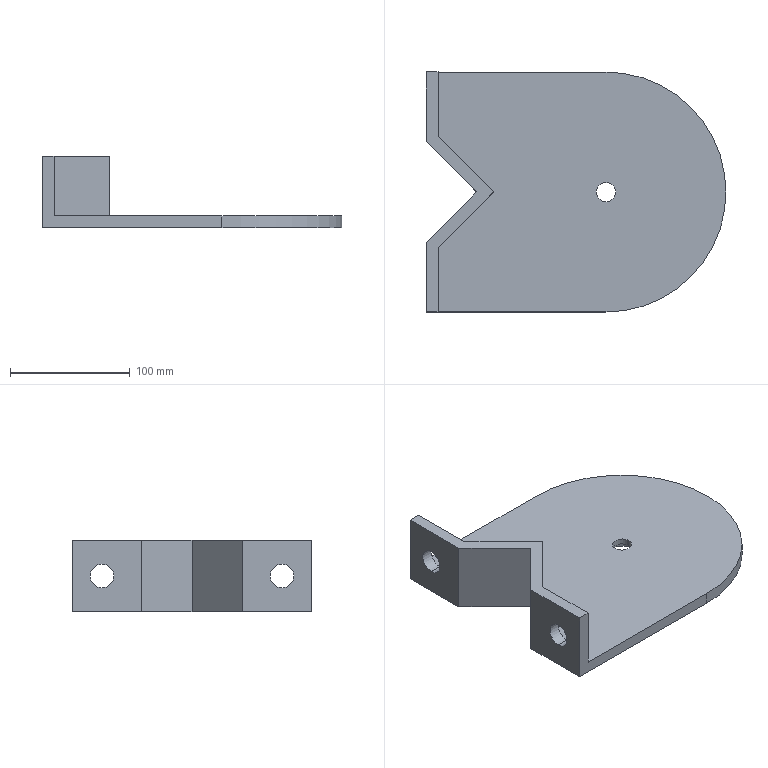Part | SolidWorks | features ICE 3, Cut 1, Extrusion 1 | 1 solid | 23 faces | box 250 x 200 x 60 mm | volume 547961 mm3 | plane 14 | cylinder 9 | commonest cylinder face diameters 20 x4 16 x2 24 x2 200 x1
STEP:
#1=CARTESIAN_POINT('',(12.,0.,5.));
#2=VERTEX_POINT('',#1);
#3=CARTESIAN_POINT('',(-12.,0.,5.));
#4=VERTEX_POINT('',#3);
#5=CARTESIAN_POINT('',(0.,0.,5.));
#6=DIRECTION('',(0.,0.,-1.));
#7=DIRECTION('',(-1.,0.,0.));
#8=AXIS2_PLACEMENT_3D('',#5,#6,#7);
#9=CIRCLE('',#8,12.);
#10=EDGE_CURVE('',#2,#4,#9,.T.);
#11=ORIENTED_EDGE('',*,*,#10,.F.);
#12=CARTESIAN_POINT('',(12.,0.,0.));
#13=VERTEX_POINT('',#12);
#14=CARTESIAN_POINT('',(12.,0.,5.));
#15=DIRECTION('',(0.,0.,-1.));
#16=VECTOR('',#15,1000.);
#17=LINE('',#14,#16);
#18=EDGE_CURVE('',#2,#13,#17,.T.);
#19=ORIENTED_EDGE('',*,*,#18,.T.);
#20=CARTESIAN_POINT('',(-12.,0.,0.));
#21=VERTEX_POINT('',#20);
#22=CARTESIAN_POINT('',(0.,0.,0.));
#23=DIRECTION('',(0.,0.,-1.));
#24=DIRECTION('',(-1.,0.,0.));
#25=AXIS2_PLACEMENT_3D('',#22,#23,#24);
#26=CIRCLE('',#25,12.);
#27=EDGE_CURVE('',#13,#21,#26,.T.);
#28=ORIENTED_EDGE('',*,*,#27,.T.);
#29=CARTESIAN_POINT('',(-12.,0.,5.));
#30=DIRECTION('',(0.,0.,-1.));
#31=VECTOR('',#30,1000.);
#32=LINE('',#29,#31);
#33=EDGE_CURVE('',#4,#21,#32,.T.);
#34=ORIENTED_EDGE('',*,*,#33,.F.);
#35=EDGE_LOOP('',(#11,#19,#28,#34));
#36=FACE_OUTER_BOUND('',#35,.T.);
#37=CARTESIAN_POINT('',(0.,0.,5.));
#38=DIRECTION('',(0.,0.,-1.));
#39=DIRECTION('',(-1.,0.,0.));
#40=AXIS2_PLACEMENT_3D('',#37,#38,#39);
#41=CYLINDRICAL_SURFACE('',#40,12.);
#42=ADVANCED_FACE('',(#36),#41,.F.);
#43=CARTESIAN_POINT('',(-140.,-75.,20.));
#44=VERTEX_POINT('',#43);
#45=CARTESIAN_POINT('',(-140.,-75.,40.));
#46=VERTEX_POINT('',#45);
#47=CARTESIAN_POINT('',(-140.,-75.,30.));
#48=DIRECTION('',(-1.,0.,0.));
#49=DIRECTION('',(0.,0.,1.));
#50=AXIS2_PLACEMENT_3D('',#47,#48,#49);
#51=CIRCLE('',#50,10.);
#52=EDGE_CURVE('',#44,#46,#51,.T.);
#53=ORIENTED_EDGE('',*,*,#52,.F.);
#54=CARTESIAN_POINT('',(-150.,-75.,20.));
#55=VERTEX_POINT('',#54);
#56=CARTESIAN_POINT('',(-110.,-75.,20.));
#57=DIRECTION('',(-1.,0.,0.));
#58=VECTOR('',#57,1000.);
#59=LINE('',#56,#58);
#60=EDGE_CURVE('',#44,#55,#59,.T.);
#61=ORIENTED_EDGE('',*,*,#60,.T.);
#62=CARTESIAN_POINT('',(-150.,-75.,40.));
#63=VERTEX_POINT('',#62);
#64=CARTESIAN_POINT('',(-150.,-75.,30.));
#65=DIRECTION('',(-1.,0.,0.));
#66=DIRECTION('',(0.,0.,1.));
#67=AXIS2_PLACEMENT_3D('',#64,#65,#66);
#68=CIRCLE('',#67,10.);
#69=EDGE_CURVE('',#55,#63,#68,.T.);
#70=ORIENTED_EDGE('',*,*,#69,.T.);
#71=CARTESIAN_POINT('',(-110.,-75.,40.));
#72=DIRECTION('',(-1.,0.,0.));
#73=VECTOR('',#72,1000.);
#74=LINE('',#71,#73);
#75=EDGE_CURVE('',#46,#63,#74,.T.);
#76=ORIENTED_EDGE('',*,*,#75,.F.);
#77=EDGE_LOOP('',(#53,#61,#70,#76));
#78=FACE_OUTER_BOUND('',#77,.T.);
#79=CARTESIAN_POINT('',(-110.,-75.,30.));
#80=DIRECTION('',(-1.,0.,0.));
#81=DIRECTION('',(0.,0.,1.));
#82=AXIS2_PLACEMENT_3D('',#79,#80,#81);
#83=CYLINDRICAL_SURFACE('',#82,10.);
#84=ADVANCED_FACE('',(#78),#83,.F.);
#85=CARTESIAN_POINT('',(-140.,75.,20.));
#86=VERTEX_POINT('',#85);
#87=CARTESIAN_POINT('',(-140.,75.,40.));
#88=VERTEX_POINT('',#87);
#89=CARTESIAN_POINT('',(-140.,75.,30.));
#90=DIRECTION('',(-1.,0.,0.));
#91=DIRECTION('',(0.,0.,1.));
#92=AXIS2_PLACEMENT_3D('',#89,#90,#91);
#93=CIRCLE('',#92,10.);
#94=EDGE_CURVE('',#86,#88,#93,.T.);
#95=ORIENTED_EDGE('',*,*,#94,.F.);
#96=CARTESIAN_POINT('',(-150.,75.,20.));
#97=VERTEX_POINT('',#96);
#98=CARTESIAN_POINT('',(-110.,75.,20.));
#99=DIRECTION('',(-1.,0.,0.));
#100=VECTOR('',#99,1000.);
#101=LINE('',#98,#100);
#102=EDGE_CURVE('',#86,#97,#101,.T.);
#103=ORIENTED_EDGE('',*,*,#102,.T.);
#104=CARTESIAN_POINT('',(-150.,75.,40.));
#105=VERTEX_POINT('',#104);
#106=CARTESIAN_POINT('',(-150.,75.,30.));
#107=DIRECTION('',(-1.,0.,0.));
#108=DIRECTION('',(0.,0.,1.));
#109=AXIS2_PLACEMENT_3D('',#106,#107,#108);
#110=CIRCLE('',#109,10.);
#111=EDGE_CURVE('',#97,#105,#110,.T.);
#112=ORIENTED_EDGE('',*,*,#111,.T.);
#113=CARTESIAN_POINT('',(-110.,75.,40.));
#114=DIRECTION('',(-1.,0.,0.));
#115=VECTOR('',#114,1000.);
#116=LINE('',#113,#115);
#117=EDGE_CURVE('',#88,#105,#116,.T.);
#118=ORIENTED_EDGE('',*,*,#117,.F.);
#119=EDGE_LOOP('',(#95,#103,#112,#118));
#120=FACE_OUTER_BOUND('',#119,.T.);
#121=CARTESIAN_POINT('',(-110.,75.,30.));
#122=DIRECTION('',(-1.,0.,0.));
#123=DIRECTION('',(0.,0.,1.));
#124=AXIS2_PLACEMENT_3D('',#121,#122,#123);
#125=CYLINDRICAL_SURFACE('',#124,10.);
#126=ADVANCED_FACE('',(#120),#125,.F.);
#127=CARTESIAN_POINT('',(-8.,0.,10.));
#128=VERTEX_POINT('',#127);
#129=CARTESIAN_POINT('',(8.,0.,10.));
#130=VERTEX_POINT('',#129);
#131=CARTESIAN_POINT('',(0.,0.,10.));
#132=DIRECTION('',(0.,0.,1.));
#133=DIRECTION('',(1.,0.,0.));
#134=AXIS2_PLACEMENT_3D('',#131,#132,#133);
#135=CIRCLE('',#134,8.);
#136=EDGE_CURVE('',#128,#130,#135,.T.);
#137=ORIENTED_EDGE('',*,*,#136,.T.);
#138=CARTESIAN_POINT('',(8.,0.,5.));
#139=VERTEX_POINT('',#138);
#140=CARTESIAN_POINT('',(8.,0.,10.));
#141=DIRECTION('',(0.,0.,-1.));
#142=VECTOR('',#141,1000.);
#143=LINE('',#140,#142);
#144=EDGE_CURVE('',#130,#139,#143,.T.);
#145=ORIENTED_EDGE('',*,*,#144,.T.);
#146=CARTESIAN_POINT('',(-8.,0.,5.));
#147=VERTEX_POINT('',#146);
#148=CARTESIAN_POINT('',(0.,0.,5.));
#149=DIRECTION('',(0.,0.,-1.));
#150=DIRECTION('',(-1.,0.,0.));
#151=AXIS2_PLACEMENT_3D('',#148,#149,#150);
#152=CIRCLE('',#151,8.);
#153=EDGE_CURVE('',#139,#147,#152,.T.);
#154=ORIENTED_EDGE('',*,*,#153,.T.);
#155=CARTESIAN_POINT('',(-8.,0.,10.));
#156=DIRECTION('',(0.,0.,-1.));
#157=VECTOR('',#156,1000.);
#158=LINE('',#155,#157);
#159=EDGE_CURVE('',#128,#147,#158,.T.);
#160=ORIENTED_EDGE('',*,*,#159,.F.);
#161=EDGE_LOOP('',(#137,#145,#154,#160));
#162=FACE_OUTER_BOUND('',#161,.T.);
#163=CARTESIAN_POINT('',(0.,0.,10.));
#164=DIRECTION('',(0.,0.,-1.));
#165=DIRECTION('',(-1.,0.,0.));
#166=AXIS2_PLACEMENT_3D('',#163,#164,#165);
#167=CYLINDRICAL_SURFACE('',#166,8.);
#168=ADVANCED_FACE('',(#162),#167,.F.);
#169=ORIENTED_EDGE('',*,*,#144,.F.);
#170=CARTESIAN_POINT('',(0.,0.,10.));
#171=DIRECTION('',(0.,0.,1.));
#172=DIRECTION('',(1.,0.,0.));
#173=AXIS2_PLACEMENT_3D('',#170,#171,#172);
#174=CIRCLE('',#173,8.);
#175=EDGE_CURVE('',#130,#128,#174,.T.);
#176=ORIENTED_EDGE('',*,*,#175,.T.);
#177=ORIENTED_EDGE('',*,*,#159,.T.);
#178=CARTESIAN_POINT('',(0.,0.,5.));
#179=DIRECTION('',(0.,0.,-1.));
#180=DIRECTION('',(-1.,0.,0.));
#181=AXIS2_PLACEMENT_3D('',#178,#179,#180);
#182=CIRCLE('',#181,8.);
#183=EDGE_CURVE('',#147,#139,#182,.T.);
#184=ORIENTED_EDGE('',*,*,#183,.T.);
#185=EDGE_LOOP('',(#169,#176,#177,#184));
#186=FACE_OUTER_BOUND('',#185,.T.);
#187=CARTESIAN_POINT('',(0.,0.,10.));
#188=DIRECTION('',(0.,0.,-1.));
#189=DIRECTION('',(-1.,0.,0.));
#190=AXIS2_PLACEMENT_3D('',#187,#188,#189);
#191=CYLINDRICAL_SURFACE('',#190,8.);
#192=ADVANCED_FACE('',(#186),#191,.F.);
#193=CARTESIAN_POINT('',(-150.,75.,30.));
#194=DIRECTION('',(-1.,0.,0.));
#195=DIRECTION('',(0.,0.,1.));
#196=AXIS2_PLACEMENT_3D('',#193,#194,#195);
#197=CIRCLE('',#196,10.);
#198=EDGE_CURVE('',#105,#97,#197,.T.);
#199=ORIENTED_EDGE('',*,*,#198,.F.);
#200=ORIENTED_EDGE('',*,*,#111,.F.);
#201=EDGE_LOOP('',(#199,#200));
#202=FACE_BOUND('',#201,.T.);
#203=CARTESIAN_POINT('',(-150.,100.,0.));
#204=VERTEX_POINT('',#203);
#205=CARTESIAN_POINT('',(-150.,42.426,0.));
#206=VERTEX_POINT('',#205);
#207=CARTESIAN_POINT('',(-150.,100.,0.));
#208=DIRECTION('',(0.,-1.,0.));
#209=VECTOR('',#208,1000.);
#210=LINE('',#207,#209);
#211=EDGE_CURVE('',#204,#206,#210,.T.);
#212=ORIENTED_EDGE('',*,*,#211,.T.);
#213=CARTESIAN_POINT('',(-150.,42.426,60.));
#214=VERTEX_POINT('',#213);
#215=CARTESIAN_POINT('',(-150.,42.426,60.));
#216=DIRECTION('',(0.,0.,-1.));
#217=VECTOR('',#216,1000.);
#218=LINE('',#215,#217);
#219=EDGE_CURVE('',#214,#206,#218,.T.);
#220=ORIENTED_EDGE('',*,*,#219,.F.);
#221=CARTESIAN_POINT('',(-150.,100.,60.));
#222=VERTEX_POINT('',#221);
#223=CARTESIAN_POINT('',(-150.,42.426,60.));
#224=DIRECTION('',(0.,-1.,0.));
#225=VECTOR('',#224,1000.);
#226=LINE('',#223,#225);
#227=EDGE_CURVE('',#222,#214,#226,.T.);
#228=ORIENTED_EDGE('',*,*,#227,.F.);
#229=CARTESIAN_POINT('',(-150.,100.,10.));
#230=DIRECTION('',(0.,0.,-1.));
#231=VECTOR('',#230,1000.);
#232=LINE('',#229,#231);
#233=EDGE_CURVE('',#222,#204,#232,.T.);
#234=ORIENTED_EDGE('',*,*,#233,.T.);
#235=EDGE_LOOP('',(#212,#220,#228,#234));
#236=FACE_OUTER_BOUND('',#235,.T.);
#237=CARTESIAN_POINT('',(-150.,100.,10.));
#238=DIRECTION('',(1.,0.,0.));
#239=DIRECTION('',(0.,1.,0.));
#240=AXIS2_PLACEMENT_3D('',#237,#238,#239);
#241=PLANE('',#240);
#242=ADVANCED_FACE('',(#202,#236),#241,.F.);
#243=CARTESIAN_POINT('',(-140.,46.569,10.));
#244=VERTEX_POINT('',#243);
#245=CARTESIAN_POINT('',(-140.,100.,10.));
#246=VERTEX_POINT('',#245);
#247=CARTESIAN_POINT('',(-140.,100.,10.));
#248=DIRECTION('',(0.,1.,0.));
#249=VECTOR('',#248,1000.);
#250=LINE('',#247,#249);
#251=EDGE_CURVE('',#244,#246,#250,.T.);
#252=ORIENTED_EDGE('',*,*,#251,.F.);
#253=CARTESIAN_POINT('',(-93.431,0.,10.));
#254=VERTEX_POINT('',#253);
#255=CARTESIAN_POINT('',(-140.,46.569,10.));
#256=DIRECTION('',(-0.7071,0.7071,0.));
#257=VECTOR('',#256,1000.);
#258=LINE('',#255,#257);
#259=EDGE_CURVE('',#254,#244,#258,.T.);
#260=ORIENTED_EDGE('',*,*,#259,.F.);
#261=CARTESIAN_POINT('',(-140.,-46.569,10.));
#262=VERTEX_POINT('',#261);
#263=CARTESIAN_POINT('',(-93.431,0.,10.));
#264=DIRECTION('',(0.7071,0.7071,0.));
#265=VECTOR('',#264,1000.);
#266=LINE('',#263,#265);
#267=EDGE_CURVE('',#262,#254,#266,.T.);
#268=ORIENTED_EDGE('',*,*,#267,.F.);
#269=CARTESIAN_POINT('',(-140.,-100.,10.));
#270=VERTEX_POINT('',#269);
#271=CARTESIAN_POINT('',(-140.,-46.569,10.));
#272=DIRECTION('',(0.,1.,0.));
#273=VECTOR('',#272,1000.);
#274=LINE('',#271,#273);
#275=EDGE_CURVE('',#270,#262,#274,.T.);
#276=ORIENTED_EDGE('',*,*,#275,.F.);
#277=CARTESIAN_POINT('',(0.,-100.,10.));
#278=VERTEX_POINT('',#277);
#279=CARTESIAN_POINT('',(-150.,-100.,10.));
#280=DIRECTION('',(1.,0.,0.));
#281=VECTOR('',#280,1000.);
#282=LINE('',#279,#281);
#283=EDGE_CURVE('',#270,#278,#282,.T.);
#284=ORIENTED_EDGE('',*,*,#283,.T.);
#285=CARTESIAN_POINT('',(0.,100.,10.));
#286=VERTEX_POINT('',#285);
#287=CARTESIAN_POINT('',(0.,0.,10.));
#288=DIRECTION('',(0.,0.,1.));
#289=DIRECTION('',(1.,0.,0.));
#290=AXIS2_PLACEMENT_3D('',#287,#288,#289);
#291=CIRCLE('',#290,100.);
#292=EDGE_CURVE('',#278,#286,#291,.T.);
#293=ORIENTED_EDGE('',*,*,#292,.T.);
#294=CARTESIAN_POINT('',(0.,100.,10.));
#295=DIRECTION('',(-1.,0.,0.));
#296=VECTOR('',#295,1000.);
#297=LINE('',#294,#296);
#298=EDGE_CURVE('',#286,#246,#297,.T.);
#299=ORIENTED_EDGE('',*,*,#298,.T.);
#300=EDGE_LOOP('',(#252,#260,#268,#276,#284,#293,#299));
#301=FACE_OUTER_BOUND('',#300,.T.);
#302=ORIENTED_EDGE('',*,*,#136,.F.);
#303=ORIENTED_EDGE('',*,*,#175,.F.);
#304=EDGE_LOOP('',(#302,#303));
#305=FACE_BOUND('',#304,.T.);
#306=CARTESIAN_POINT('',(0.,0.,10.));
#307=DIRECTION('',(0.,0.,1.));
#308=DIRECTION('',(1.,0.,0.));
#309=AXIS2_PLACEMENT_3D('',#306,#307,#308);
#310=PLANE('',#309);
#311=ADVANCED_FACE('',(#301,#305),#310,.T.);
#312=CARTESIAN_POINT('',(0.,0.,0.));
#313=DIRECTION('',(0.,0.,-1.));
#314=DIRECTION('',(-1.,0.,0.));
#315=AXIS2_PLACEMENT_3D('',#312,#313,#314);
#316=CIRCLE('',#315,12.);
#317=EDGE_CURVE('',#21,#13,#316,.T.);
#318=ORIENTED_EDGE('',*,*,#317,.F.);
#319=ORIENTED_EDGE('',*,*,#27,.F.);
#320=EDGE_LOOP('',(#318,#319));
#321=FACE_BOUND('',#320,.T.);
#322=CARTESIAN_POINT('',(-150.,-42.426,0.));
#323=VERTEX_POINT('',#322);
#324=CARTESIAN_POINT('',(-107.574,0.,0.));
#325=VERTEX_POINT('',#324);
#326=CARTESIAN_POINT('',(-150.,-42.426,0.));
#327=DIRECTION('',(0.7071,0.7071,0.));
#328=VECTOR('',#327,1000.);
#329=LINE('',#326,#328);
#330=EDGE_CURVE('',#323,#325,#329,.T.);
#331=ORIENTED_EDGE('',*,*,#330,.T.);
#332=CARTESIAN_POINT('',(-107.574,0.,0.));
#333=DIRECTION('',(-0.7071,0.7071,0.));
#334=VECTOR('',#333,1000.);
#335=LINE('',#332,#334);
#336=EDGE_CURVE('',#325,#206,#335,.T.);
#337=ORIENTED_EDGE('',*,*,#336,.T.);
#338=ORIENTED_EDGE('',*,*,#211,.F.);
#339=CARTESIAN_POINT('',(0.,100.,0.));
#340=VERTEX_POINT('',#339);
#341=CARTESIAN_POINT('',(0.,100.,0.));
#342=DIRECTION('',(-1.,0.,0.));
#343=VECTOR('',#342,1000.);
#344=LINE('',#341,#343);
#345=EDGE_CURVE('',#340,#204,#344,.T.);
#346=ORIENTED_EDGE('',*,*,#345,.F.);
#347=CARTESIAN_POINT('',(0.,-100.,0.));
#348=VERTEX_POINT('',#347);
#349=CARTESIAN_POINT('',(0.,0.,0.));
#350=DIRECTION('',(0.,0.,1.));
#351=DIRECTION('',(1.,0.,0.));
#352=AXIS2_PLACEMENT_3D('',#349,#350,#351);
#353=CIRCLE('',#352,100.);
#354=EDGE_CURVE('',#348,#340,#353,.T.);
#355=ORIENTED_EDGE('',*,*,#354,.F.);
#356=CARTESIAN_POINT('',(-150.,-100.,0.));
#357=VERTEX_POINT('',#356);
#358=CARTESIAN_POINT('',(-150.,-100.,0.));
#359=DIRECTION('',(1.,0.,0.));
#360=VECTOR('',#359,1000.);
#361=LINE('',#358,#360);
#362=EDGE_CURVE('',#357,#348,#361,.T.);
#363=ORIENTED_EDGE('',*,*,#362,.F.);
#364=CARTESIAN_POINT('',(-150.,100.,0.));
#365=DIRECTION('',(0.,-1.,0.));
#366=VECTOR('',#365,1000.);
#367=LINE('',#364,#366);
#368=EDGE_CURVE('',#323,#357,#367,.T.);
#369=ORIENTED_EDGE('',*,*,#368,.F.);
#370=EDGE_LOOP('',(#331,#337,#338,#346,#355,#363,#369));
#371=FACE_OUTER_BOUND('',#370,.T.);
#372=CARTESIAN_POINT('',(0.,0.,0.));
#373=DIRECTION('',(0.,0.,1.));
#374=DIRECTION('',(1.,0.,0.));
#375=AXIS2_PLACEMENT_3D('',#372,#373,#374);
#376=PLANE('',#375);
#377=ADVANCED_FACE('',(#321,#371),#376,.F.);
#378=ORIENTED_EDGE('',*,*,#354,.T.);
#379=CARTESIAN_POINT('',(0.,100.,10.));
#380=DIRECTION('',(0.,0.,-1.));
#381=VECTOR('',#380,1000.);
#382=LINE('',#379,#381);
#383=EDGE_CURVE('',#286,#340,#382,.T.);
#384=ORIENTED_EDGE('',*,*,#383,.F.);
#385=ORIENTED_EDGE('',*,*,#292,.F.);
#386=CARTESIAN_POINT('',(0.,-100.,10.));
#387=DIRECTION('',(0.,0.,-1.));
#388=VECTOR('',#387,1000.);
#389=LINE('',#386,#388);
#390=EDGE_CURVE('',#278,#348,#389,.T.);
#391=ORIENTED_EDGE('',*,*,#390,.T.);
#392=EDGE_LOOP('',(#378,#384,#385,#391));
#393=FACE_OUTER_BOUND('',#392,.T.);
#394=CARTESIAN_POINT('',(0.,0.,10.));
#395=DIRECTION('',(0.,0.,-1.));
#396=DIRECTION('',(-1.,0.,0.));
#397=AXIS2_PLACEMENT_3D('',#394,#395,#396);
#398=CYLINDRICAL_SURFACE('',#397,100.);
#399=ADVANCED_FACE('',(#393),#398,.T.);
#400=ORIENTED_EDGE('',*,*,#345,.T.);
#401=ORIENTED_EDGE('',*,*,#233,.F.);
#402=CARTESIAN_POINT('',(-140.,100.,60.));
#403=VERTEX_POINT('',#402);
#404=CARTESIAN_POINT('',(-150.,100.,60.));
#405=DIRECTION('',(-1.,0.,0.));
#406=VECTOR('',#405,1000.);
#407=LINE('',#404,#406);
#408=EDGE_CURVE('',#403,#222,#407,.T.);
#409=ORIENTED_EDGE('',*,*,#408,.F.);
#410=CARTESIAN_POINT('',(-140.,100.,60.));
#411=DIRECTION('',(0.,0.,-1.));
#412=VECTOR('',#411,1000.);
#413=LINE('',#410,#412);
#414=EDGE_CURVE('',#403,#246,#413,.T.);
#415=ORIENTED_EDGE('',*,*,#414,.T.);
#416=ORIENTED_EDGE('',*,*,#298,.F.);
#417=ORIENTED_EDGE('',*,*,#383,.T.);
#418=EDGE_LOOP('',(#400,#401,#409,#415,#416,#417));
#419=FACE_OUTER_BOUND('',#418,.T.);
#420=CARTESIAN_POINT('',(0.,100.,10.));
#421=DIRECTION('',(0.,-1.,0.));
#422=DIRECTION('',(1.,0.,0.));
#423=AXIS2_PLACEMENT_3D('',#420,#421,#422);
#424=PLANE('',#423);
#425=ADVANCED_FACE('',(#419),#424,.F.);
#426=CARTESIAN_POINT('',(-150.,-75.,30.));
#427=DIRECTION('',(-1.,0.,0.));
#428=DIRECTION('',(0.,0.,1.));
#429=AXIS2_PLACEMENT_3D('',#426,#427,#428);
#430=CIRCLE('',#429,10.);
#431=EDGE_CURVE('',#63,#55,#430,.T.);
#432=ORIENTED_EDGE('',*,*,#431,.F.);
#433=ORIENTED_EDGE('',*,*,#69,.F.);
#434=EDGE_LOOP('',(#432,#433));
#435=FACE_BOUND('',#434,.T.);
#436=CARTESIAN_POINT('',(-150.,-42.426,60.));
#437=VERTEX_POINT('',#436);
#438=CARTESIAN_POINT('',(-150.,-42.426,60.));
#439=DIRECTION('',(0.,0.,-1.));
#440=VECTOR('',#439,1000.);
#441=LINE('',#438,#440);
#442=EDGE_CURVE('',#437,#323,#441,.T.);
#443=ORIENTED_EDGE('',*,*,#442,.T.);
#444=ORIENTED_EDGE('',*,*,#368,.T.);
#445=CARTESIAN_POINT('',(-150.,-100.,60.));
#446=VERTEX_POINT('',#445);
#447=CARTESIAN_POINT('',(-150.,-100.,10.));
#448=DIRECTION('',(0.,0.,-1.));
#449=VECTOR('',#448,1000.);
#450=LINE('',#447,#449);
#451=EDGE_CURVE('',#446,#357,#450,.T.);
#452=ORIENTED_EDGE('',*,*,#451,.F.);
#453=CARTESIAN_POINT('',(-150.,-100.,60.));
#454=DIRECTION('',(0.,-1.,0.));
#455=VECTOR('',#454,1000.);
#456=LINE('',#453,#455);
#457=EDGE_CURVE('',#437,#446,#456,.T.);
#458=ORIENTED_EDGE('',*,*,#457,.F.);
#459=EDGE_LOOP('',(#443,#444,#452,#458));
#460=FACE_OUTER_BOUND('',#459,.T.);
#461=CARTESIAN_POINT('',(-150.,100.,10.));
#462=DIRECTION('',(1.,0.,0.));
#463=DIRECTION('',(0.,1.,0.));
#464=AXIS2_PLACEMENT_3D('',#461,#462,#463);
#465=PLANE('',#464);
#466=ADVANCED_FACE('',(#435,#460),#465,.F.);
#467=ORIENTED_EDGE('',*,*,#362,.T.);
#468=ORIENTED_EDGE('',*,*,#390,.F.);
#469=ORIENTED_EDGE('',*,*,#283,.F.);
#470=CARTESIAN_POINT('',(-140.,-100.,60.));
#471=VERTEX_POINT('',#470);
#472=CARTESIAN_POINT('',(-140.,-100.,60.));
#473=DIRECTION('',(0.,0.,-1.));
#474=VECTOR('',#473,1000.);
#475=LINE('',#472,#474);
#476=EDGE_CURVE('',#471,#270,#475,.T.);
#477=ORIENTED_EDGE('',*,*,#476,.F.);
#478=CARTESIAN_POINT('',(-140.,-100.,60.));
#479=DIRECTION('',(1.,0.,0.));
#480=VECTOR('',#479,1000.);
#481=LINE('',#478,#480);
#482=EDGE_CURVE('',#446,#471,#481,.T.);
#483=ORIENTED_EDGE('',*,*,#482,.F.);
#484=ORIENTED_EDGE('',*,*,#451,.T.);
#485=EDGE_LOOP('',(#467,#468,#469,#477,#483,#484));
#486=FACE_OUTER_BOUND('',#485,.T.);
#487=CARTESIAN_POINT('',(-150.,-100.,10.));
#488=DIRECTION('',(0.,1.,0.));
#489=DIRECTION('',(-1.,0.,0.));
#490=AXIS2_PLACEMENT_3D('',#487,#488,#489);
#491=PLANE('',#490);
#492=ADVANCED_FACE('',(#486),#491,.F.);
#493=ORIENTED_EDGE('',*,*,#219,.T.);
#494=ORIENTED_EDGE('',*,*,#336,.F.);
#495=CARTESIAN_POINT('',(-107.574,0.,60.));
#496=VERTEX_POINT('',#495);
#497=CARTESIAN_POINT('',(-107.574,0.,60.));
#498=DIRECTION('',(0.,0.,-1.));
#499=VECTOR('',#498,1000.);
#500=LINE('',#497,#499);
#501=EDGE_CURVE('',#496,#325,#500,.T.);
#502=ORIENTED_EDGE('',*,*,#501,.F.);
#503=CARTESIAN_POINT('',(-150.,42.426,60.));
#504=DIRECTION('',(0.7071,-0.7071,0.));
#505=VECTOR('',#504,1000.);
#506=LINE('',#503,#505);
#507=EDGE_CURVE('',#214,#496,#506,.T.);
#508=ORIENTED_EDGE('',*,*,#507,.F.);
#509=EDGE_LOOP('',(#493,#494,#502,#508));
#510=FACE_OUTER_BOUND('',#509,.T.);
#511=CARTESIAN_POINT('',(-150.,42.426,60.));
#512=DIRECTION('',(0.7071,0.7071,0.));
#513=DIRECTION('',(-0.7071,0.7071,0.));
#514=AXIS2_PLACEMENT_3D('',#511,#512,#513);
#515=PLANE('',#514);
#516=ADVANCED_FACE('',(#510),#515,.F.);
#517=ORIENTED_EDGE('',*,*,#501,.T.);
#518=ORIENTED_EDGE('',*,*,#330,.F.);
#519=ORIENTED_EDGE('',*,*,#442,.F.);
#520=CARTESIAN_POINT('',(-107.574,0.,60.));
#521=DIRECTION('',(-0.7071,-0.7071,0.));
#522=VECTOR('',#521,1000.);
#523=LINE('',#520,#522);
#524=EDGE_CURVE('',#496,#437,#523,.T.);
#525=ORIENTED_EDGE('',*,*,#524,.F.);
#526=EDGE_LOOP('',(#517,#518,#519,#525));
#527=FACE_OUTER_BOUND('',#526,.T.);
#528=CARTESIAN_POINT('',(-107.574,0.,60.));
#529=DIRECTION('',(0.7071,-0.7071,0.));
#530=DIRECTION('',(0.7071,0.7071,0.));
#531=AXIS2_PLACEMENT_3D('',#528,#529,#530);
#532=PLANE('',#531);
#533=ADVANCED_FACE('',(#527),#532,.F.);
#534=CARTESIAN_POINT('',(-140.,-75.,30.));
#535=DIRECTION('',(-1.,0.,0.));
#536=DIRECTION('',(0.,0.,1.));
#537=AXIS2_PLACEMENT_3D('',#534,#535,#536);
#538=CIRCLE('',#537,10.);
#539=EDGE_CURVE('',#46,#44,#538,.T.);
#540=ORIENTED_EDGE('',*,*,#539,.T.);
#541=ORIENTED_EDGE('',*,*,#52,.T.);
#542=EDGE_LOOP('',(#540,#541));
#543=FACE_BOUND('',#542,.T.);
#544=ORIENTED_EDGE('',*,*,#275,.T.);
#545=CARTESIAN_POINT('',(-140.,-46.569,60.));
#546=VERTEX_POINT('',#545);
#547=CARTESIAN_POINT('',(-140.,-46.569,60.));
#548=DIRECTION('',(0.,0.,-1.));
#549=VECTOR('',#548,1000.);
#550=LINE('',#547,#549);
#551=EDGE_CURVE('',#546,#262,#550,.T.);
#552=ORIENTED_EDGE('',*,*,#551,.F.);
#553=CARTESIAN_POINT('',(-140.,-46.569,60.));
#554=DIRECTION('',(0.,1.,0.));
#555=VECTOR('',#554,1000.);
#556=LINE('',#553,#555);
#557=EDGE_CURVE('',#471,#546,#556,.T.);
#558=ORIENTED_EDGE('',*,*,#557,.F.);
#559=ORIENTED_EDGE('',*,*,#476,.T.);
#560=EDGE_LOOP('',(#544,#552,#558,#559));
#561=FACE_OUTER_BOUND('',#560,.T.);
#562=CARTESIAN_POINT('',(-140.,-46.569,60.));
#563=DIRECTION('',(-1.,0.,0.));
#564=DIRECTION('',(0.,0.,1.));
#565=AXIS2_PLACEMENT_3D('',#562,#563,#564);
#566=PLANE('',#565);
#567=ADVANCED_FACE('',(#543,#561),#566,.F.);
#568=ORIENTED_EDGE('',*,*,#267,.T.);
#569=CARTESIAN_POINT('',(-93.431,0.,60.));
#570=VERTEX_POINT('',#569);
#571=CARTESIAN_POINT('',(-93.431,0.,60.));
#572=DIRECTION('',(0.,0.,-1.));
#573=VECTOR('',#572,1000.);
#574=LINE('',#571,#573);
#575=EDGE_CURVE('',#570,#254,#574,.T.);
#576=ORIENTED_EDGE('',*,*,#575,.F.);
#577=CARTESIAN_POINT('',(-93.431,0.,60.));
#578=DIRECTION('',(0.7071,0.7071,0.));
#579=VECTOR('',#578,1000.);
#580=LINE('',#577,#579);
#581=EDGE_CURVE('',#546,#570,#580,.T.);
#582=ORIENTED_EDGE('',*,*,#581,.F.);
#583=ORIENTED_EDGE('',*,*,#551,.T.);
#584=EDGE_LOOP('',(#568,#576,#582,#583));
#585=FACE_OUTER_BOUND('',#584,.T.);
#586=CARTESIAN_POINT('',(-93.431,0.,60.));
#587=DIRECTION('',(-0.7071,0.7071,0.));
#588=DIRECTION('',(-0.7071,-0.7071,0.));
#589=AXIS2_PLACEMENT_3D('',#586,#587,#588);
#590=PLANE('',#589);
#591=ADVANCED_FACE('',(#585),#590,.F.);
#592=ORIENTED_EDGE('',*,*,#259,.T.);
#593=CARTESIAN_POINT('',(-140.,46.569,60.));
#594=VERTEX_POINT('',#593);
#595=CARTESIAN_POINT('',(-140.,46.569,60.));
#596=DIRECTION('',(0.,0.,-1.));
#597=VECTOR('',#596,1000.);
#598=LINE('',#595,#597);
#599=EDGE_CURVE('',#594,#244,#598,.T.);
#600=ORIENTED_EDGE('',*,*,#599,.F.);
#601=CARTESIAN_POINT('',(-140.,46.569,60.));
#602=DIRECTION('',(-0.7071,0.7071,0.));
#603=VECTOR('',#602,1000.);
#604=LINE('',#601,#603);
#605=EDGE_CURVE('',#570,#594,#604,.T.);
#606=ORIENTED_EDGE('',*,*,#605,.F.);
#607=ORIENTED_EDGE('',*,*,#575,.T.);
#608=EDGE_LOOP('',(#592,#600,#606,#607));
#609=FACE_OUTER_BOUND('',#608,.T.);
#610=CARTESIAN_POINT('',(-140.,46.569,60.));
#611=DIRECTION('',(-0.7071,-0.7071,0.));
#612=DIRECTION('',(0.7071,-0.7071,0.));
#613=AXIS2_PLACEMENT_3D('',#610,#611,#612);
#614=PLANE('',#613);
#615=ADVANCED_FACE('',(#609),#614,.F.);
#616=CARTESIAN_POINT('',(-140.,75.,30.));
#617=DIRECTION('',(-1.,0.,0.));
#618=DIRECTION('',(0.,0.,1.));
#619=AXIS2_PLACEMENT_3D('',#616,#617,#618);
#620=CIRCLE('',#619,10.);
#621=EDGE_CURVE('',#88,#86,#620,.T.);
#622=ORIENTED_EDGE('',*,*,#621,.T.);
#623=ORIENTED_EDGE('',*,*,#94,.T.);
#624=EDGE_LOOP('',(#622,#623));
#625=FACE_BOUND('',#624,.T.);
#626=ORIENTED_EDGE('',*,*,#251,.T.);
#627=ORIENTED_EDGE('',*,*,#414,.F.);
#628=CARTESIAN_POINT('',(-140.,100.,60.));
#629=DIRECTION('',(0.,1.,0.));
#630=VECTOR('',#629,1000.);
#631=LINE('',#628,#630);
#632=EDGE_CURVE('',#594,#403,#631,.T.);
#633=ORIENTED_EDGE('',*,*,#632,.F.);
#634=ORIENTED_EDGE('',*,*,#599,.T.);
#635=EDGE_LOOP('',(#626,#627,#633,#634));
#636=FACE_OUTER_BOUND('',#635,.T.);
#637=CARTESIAN_POINT('',(-140.,100.,60.));
#638=DIRECTION('',(-1.,0.,0.));
#639=DIRECTION('',(0.,0.,1.));
#640=AXIS2_PLACEMENT_3D('',#637,#638,#639);
#641=PLANE('',#640);
#642=ADVANCED_FACE('',(#625,#636),#641,.F.);
#643=ORIENTED_EDGE('',*,*,#408,.T.);
#644=ORIENTED_EDGE('',*,*,#227,.T.);
#645=ORIENTED_EDGE('',*,*,#507,.T.);
#646=ORIENTED_EDGE('',*,*,#524,.T.);
#647=ORIENTED_EDGE('',*,*,#457,.T.);
#648=ORIENTED_EDGE('',*,*,#482,.T.);
#649=ORIENTED_EDGE('',*,*,#557,.T.);
#650=ORIENTED_EDGE('',*,*,#581,.T.);
#651=ORIENTED_EDGE('',*,*,#605,.T.);
#652=ORIENTED_EDGE('',*,*,#632,.T.);
#653=EDGE_LOOP('',(#643,#644,#645,#646,#647,#648,#649,#650,#651,#652));
#654=FACE_OUTER_BOUND('',#653,.T.);
#655=CARTESIAN_POINT('',(0.,0.,60.));
#656=DIRECTION('',(0.,0.,-1.));
#657=DIRECTION('',(-1.,0.,0.));
#658=AXIS2_PLACEMENT_3D('',#655,#656,#657);
#659=PLANE('',#658);
#660=ADVANCED_FACE('',(#654),#659,.F.);
#661=ORIENTED_EDGE('',*,*,#102,.F.);
#662=ORIENTED_EDGE('',*,*,#621,.F.);
#663=ORIENTED_EDGE('',*,*,#117,.T.);
#664=ORIENTED_EDGE('',*,*,#198,.T.);
#665=EDGE_LOOP('',(#661,#662,#663,#664));
#666=FACE_OUTER_BOUND('',#665,.T.);
#667=CARTESIAN_POINT('',(-110.,75.,30.));
#668=DIRECTION('',(-1.,0.,0.));
#669=DIRECTION('',(0.,0.,1.));
#670=AXIS2_PLACEMENT_3D('',#667,#668,#669);
#671=CYLINDRICAL_SURFACE('',#670,10.);
#672=ADVANCED_FACE('',(#666),#671,.F.);
#673=ORIENTED_EDGE('',*,*,#60,.F.);
#674=ORIENTED_EDGE('',*,*,#539,.F.);
#675=ORIENTED_EDGE('',*,*,#75,.T.);
#676=ORIENTED_EDGE('',*,*,#431,.T.);
#677=EDGE_LOOP('',(#673,#674,#675,#676));
#678=FACE_OUTER_BOUND('',#677,.T.);
#679=CARTESIAN_POINT('',(-110.,-75.,30.));
#680=DIRECTION('',(-1.,0.,0.));
#681=DIRECTION('',(0.,0.,1.));
#682=AXIS2_PLACEMENT_3D('',#679,#680,#681);
#683=CYLINDRICAL_SURFACE('',#682,10.);
#684=ADVANCED_FACE('',(#678),#683,.F.);
#685=ORIENTED_EDGE('',*,*,#18,.F.);
#686=CARTESIAN_POINT('',(0.,0.,5.));
#687=DIRECTION('',(0.,0.,-1.));
#688=DIRECTION('',(-1.,0.,0.));
#689=AXIS2_PLACEMENT_3D('',#686,#687,#688);
#690=CIRCLE('',#689,12.);
#691=EDGE_CURVE('',#4,#2,#690,.T.);
#692=ORIENTED_EDGE('',*,*,#691,.F.);
#693=ORIENTED_EDGE('',*,*,#33,.T.);
#694=ORIENTED_EDGE('',*,*,#317,.T.);
#695=EDGE_LOOP('',(#685,#692,#693,#694));
#696=FACE_OUTER_BOUND('',#695,.T.);
#697=CARTESIAN_POINT('',(0.,0.,5.));
#698=DIRECTION('',(0.,0.,-1.));
#699=DIRECTION('',(-1.,0.,0.));
#700=AXIS2_PLACEMENT_3D('',#697,#698,#699);
#701=CYLINDRICAL_SURFACE('',#700,12.);
#702=ADVANCED_FACE('',(#696),#701,.F.);
#703=ORIENTED_EDGE('',*,*,#183,.F.);
#704=ORIENTED_EDGE('',*,*,#153,.F.);
#705=EDGE_LOOP('',(#703,#704));
#706=FACE_BOUND('',#705,.T.);
#707=ORIENTED_EDGE('',*,*,#691,.T.);
#708=ORIENTED_EDGE('',*,*,#10,.T.);
#709=EDGE_LOOP('',(#707,#708));
#710=FACE_OUTER_BOUND('',#709,.T.);
#711=CARTESIAN_POINT('',(0.,0.,5.));
#712=DIRECTION('',(0.,0.,-1.));
#713=DIRECTION('',(-1.,0.,0.));
#714=AXIS2_PLACEMENT_3D('',#711,#712,#713);
#715=PLANE('',#714);
#716=ADVANCED_FACE('',(#706,#710),#715,.T.);
#717=CLOSED_SHELL('',(#42,#84,#126,#168,#192,#242,#311,#377,#399,#425,#466,#492,#516,#533,#567,#591,#615,#642,#660,#672,#684,#702,#716));
#718=MANIFOLD_SOLID_BREP('',#717);
#719=CARTESIAN_POINT('',(0.,0.,0.));
#720=DIRECTION('',(0.,0.,1.));
#721=DIRECTION('',(1.,0.,0.));
#722=AXIS2_PLACEMENT_3D('',#719,#720,#721);
#723=(LENGTH_UNIT()NAMED_UNIT(*)SI_UNIT(.MILLI.,.METRE.));
#724=UNCERTAINTY_MEASURE_WITH_UNIT(LENGTH_MEASURE(0.00001),#723,'','');
#725=(NAMED_UNIT(*)PLANE_ANGLE_UNIT()SI_UNIT($,.RADIAN.));
#726=(NAMED_UNIT(*)SI_UNIT($,.STERADIAN.)SOLID_ANGLE_UNIT());
#727=(GEOMETRIC_REPRESENTATION_CONTEXT(3)GLOBAL_UNCERTAINTY_ASSIGNED_CONTEXT((#724))GLOBAL_UNIT_ASSIGNED_CONTEXT((#723,#725,#726))REPRESENTATION_CONTEXT('',''));
#728=ADVANCED_BREP_SHAPE_REPRESENTATION('',(#718,#722),#727);